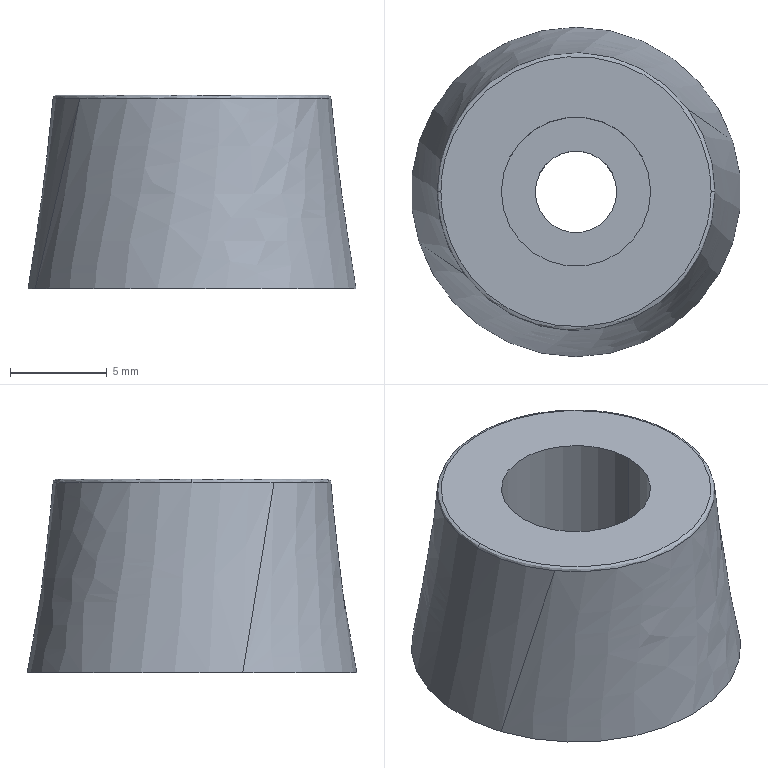Part | SolidWorks | features BaseBody 1 | 1 solid | 11 faces | box 17 x 17 x 10 mm | volume 1547 mm3 | spline 4 | cylinder 4 | plane 3 | commonest cylinder face diameters 4.2 x2 7.7 x2
STEP:
#1=CARTESIAN_POINT('',(6.967,0.,10.));
#2=VERTEX_POINT('',#1);
#3=CARTESIAN_POINT('',(-6.967,0.,10.));
#4=VERTEX_POINT('',#3);
#5=CARTESIAN_POINT('',(6.967,0.,10.));
#6=CARTESIAN_POINT('',(6.967,-13.935,10.));
#7=CARTESIAN_POINT('',(-6.967,-13.935,10.));
#8=CARTESIAN_POINT('',(-6.967,0.,10.));
#9=(BOUNDED_CURVE()B_SPLINE_CURVE(3,(#5,#6,#7,#8),.UNSPECIFIED.,.F.,.F.)B_SPLINE_CURVE_WITH_KNOTS((4,4),(0.,1.),.UNSPECIFIED.)CURVE()GEOMETRIC_REPRESENTATION_ITEM()RATIONAL_B_SPLINE_CURVE((1.,0.3333,0.3333,1.))REPRESENTATION_ITEM(''));
#10=EDGE_CURVE('',#2,#4,#9,.T.);
#11=ORIENTED_EDGE('',*,*,#10,.T.);
#12=CARTESIAN_POINT('',(-7.167,0.,9.818));
#13=VERTEX_POINT('',#12);
#14=CARTESIAN_POINT('',(-6.967,0.,9.8));
#15=DIRECTION('',(0.,-1.,0.));
#16=DIRECTION('',(-1.,0.,0.));
#17=AXIS2_PLACEMENT_3D('',#14,#15,#16);
#18=CIRCLE('',#17,0.2);
#19=EDGE_CURVE('',#4,#13,#18,.T.);
#20=ORIENTED_EDGE('',*,*,#19,.T.);
#21=CARTESIAN_POINT('',(-5.784,-4.231,9.818));
#22=VERTEX_POINT('',#21);
#23=CARTESIAN_POINT('',(0.,0.,9.818));
#24=DIRECTION('',(0.,0.,-1.));
#25=DIRECTION('',(-0.8071,-0.5904,0.));
#26=AXIS2_PLACEMENT_3D('',#23,#24,#25);
#27=CIRCLE('',#26,7.167);
#28=EDGE_CURVE('',#22,#13,#27,.T.);
#29=ORIENTED_EDGE('',*,*,#28,.F.);
#30=CARTESIAN_POINT('',(7.167,0.,9.818));
#31=VERTEX_POINT('',#30);
#32=CARTESIAN_POINT('',(0.,0.,9.818));
#33=DIRECTION('',(0.,0.,-1.));
#34=DIRECTION('',(-0.8071,-0.5904,0.));
#35=AXIS2_PLACEMENT_3D('',#32,#33,#34);
#36=CIRCLE('',#35,7.167);
#37=EDGE_CURVE('',#31,#22,#36,.T.);
#38=ORIENTED_EDGE('',*,*,#37,.F.);
#39=CARTESIAN_POINT('',(6.967,0.,9.8));
#40=DIRECTION('',(0.,1.,0.));
#41=DIRECTION('',(1.,0.,0.));
#42=AXIS2_PLACEMENT_3D('',#39,#40,#41);
#43=CIRCLE('',#42,0.2);
#44=EDGE_CURVE('',#2,#31,#43,.T.);
#45=ORIENTED_EDGE('',*,*,#44,.F.);
#46=EDGE_LOOP('',(#11,#20,#29,#38,#45));
#47=FACE_OUTER_BOUND('',#46,.T.);
#48=CARTESIAN_POINT('',(-6.967,0.,10.));
#49=CARTESIAN_POINT('',(-6.967,-13.935,10.));
#50=CARTESIAN_POINT('',(6.967,-13.935,10.));
#51=CARTESIAN_POINT('',(6.967,0.,10.));
#52=CARTESIAN_POINT('',(-7.076,0.,10.));
#53=CARTESIAN_POINT('',(-7.076,-14.152,10.));
#54=CARTESIAN_POINT('',(7.076,-14.152,10.));
#55=CARTESIAN_POINT('',(7.076,0.,10.));
#56=CARTESIAN_POINT('',(-7.157,0.,9.927));
#57=CARTESIAN_POINT('',(-7.157,-14.313,9.927));
#58=CARTESIAN_POINT('',(7.157,-14.313,9.927));
#59=CARTESIAN_POINT('',(7.157,0.,9.927));
#60=CARTESIAN_POINT('',(-7.167,0.,9.818));
#61=CARTESIAN_POINT('',(-7.167,-14.333,9.818));
#62=CARTESIAN_POINT('',(7.167,-14.333,9.818));
#63=CARTESIAN_POINT('',(7.167,0.,9.818));
#64=(BOUNDED_SURFACE()B_SPLINE_SURFACE(3,3,((#48,#49,#50,#51),(#52,#53,#54,#55),(#56,#57,#58,#59),(#60,#61,#62,#63)),.UNSPECIFIED.,.F.,.F.,.F.)B_SPLINE_SURFACE_WITH_KNOTS((4,4),(4,4),(0.,1.),(0.,1.),.UNSPECIFIED.)GEOMETRIC_REPRESENTATION_ITEM()RATIONAL_B_SPLINE_SURFACE(((1.,0.3333,0.3333,1.),(0.8259,0.2753,0.2753,0.8259),(0.8259,0.2753,0.2753,0.8259),(1.,0.3333,0.3333,1.)))REPRESENTATION_ITEM('')SURFACE());
#65=ADVANCED_FACE('',(#47),#64,.T.);
#66=CARTESIAN_POINT('',(-8.086,-2.622,0.));
#67=VERTEX_POINT('',#66);
#68=CARTESIAN_POINT('',(8.086,2.622,0.));
#69=VERTEX_POINT('',#68);
#70=CARTESIAN_POINT('',(0.,0.,0.));
#71=DIRECTION('',(0.,0.,1.));
#72=DIRECTION('',(1.,0.,0.));
#73=AXIS2_PLACEMENT_3D('',#70,#71,#72);
#74=CIRCLE('',#73,8.5);
#75=EDGE_CURVE('',#67,#69,#74,.T.);
#76=ORIENTED_EDGE('',*,*,#75,.T.);
#77=CARTESIAN_POINT('',(5.784,4.231,9.818));
#78=VERTEX_POINT('',#77);
#79=CARTESIAN_POINT('',(8.086,2.622,0.));
#80=CARTESIAN_POINT('',(5.784,4.231,9.818));
#81=B_SPLINE_CURVE_WITH_KNOTS('',1,(#79,#80),.UNSPECIFIED.,.F.,.F.,(2,2),(0.,0.9818),.UNSPECIFIED.);
#82=EDGE_CURVE('',#69,#78,#81,.T.);
#83=ORIENTED_EDGE('',*,*,#82,.T.);
#84=CARTESIAN_POINT('',(0.,0.,9.818));
#85=DIRECTION('',(0.,0.,-1.));
#86=DIRECTION('',(-0.8071,-0.5904,0.));
#87=AXIS2_PLACEMENT_3D('',#84,#85,#86);
#88=CIRCLE('',#87,7.167);
#89=EDGE_CURVE('',#78,#31,#88,.T.);
#90=ORIENTED_EDGE('',*,*,#89,.T.);
#91=ORIENTED_EDGE('',*,*,#37,.T.);
#92=CARTESIAN_POINT('',(-8.086,-2.622,0.));
#93=CARTESIAN_POINT('',(-5.784,-4.231,9.818));
#94=B_SPLINE_CURVE_WITH_KNOTS('',1,(#92,#93),.UNSPECIFIED.,.F.,.F.,(2,2),(0.,0.9818),.UNSPECIFIED.);
#95=EDGE_CURVE('',#67,#22,#94,.T.);
#96=ORIENTED_EDGE('',*,*,#95,.F.);
#97=EDGE_LOOP('',(#76,#83,#90,#91,#96));
#98=FACE_OUTER_BOUND('',#97,.T.);
#99=CARTESIAN_POINT('',(-8.086,-2.622,0.));
#100=CARTESIAN_POINT('',(-5.742,-4.261,10.));
#101=CARTESIAN_POINT('',(-2.842,-18.793,0.));
#102=CARTESIAN_POINT('',(2.779,-15.744,10.));
#103=CARTESIAN_POINT('',(13.329,-13.55,0.));
#104=CARTESIAN_POINT('',(14.263,-7.223,10.));
#105=CARTESIAN_POINT('',(8.086,2.622,0.));
#106=CARTESIAN_POINT('',(5.742,4.261,10.));
#107=CARTESIAN_POINT('',(2.842,18.793,0.));
#108=CARTESIAN_POINT('',(-2.779,15.744,10.));
#109=CARTESIAN_POINT('',(-13.329,13.55,0.));
#110=CARTESIAN_POINT('',(-14.263,7.223,10.));
#111=CARTESIAN_POINT('',(-8.086,-2.622,0.));
#112=CARTESIAN_POINT('',(-5.742,-4.261,10.));
#113=(BOUNDED_SURFACE()B_SPLINE_SURFACE(3,1,((#99,#100),(#101,#102),(#103,#104),(#105,#106),(#107,#108),(#109,#110),(#111,#112)),.UNSPECIFIED.,.T.,.F.,.F.)B_SPLINE_SURFACE_WITH_KNOTS((4,3,4),(2,2),(0.,0.5,1.),(0.,1.),.UNSPECIFIED.)GEOMETRIC_REPRESENTATION_ITEM()RATIONAL_B_SPLINE_SURFACE(((1.,1.),(0.3333,0.3333),(0.3333,0.3333),(1.,1.),(0.3333,0.3333),(0.3333,0.3333),(1.,1.)))REPRESENTATION_ITEM('')SURFACE());
#114=ADVANCED_FACE('',(#98),#113,.T.);
#115=CARTESIAN_POINT('',(2.1,0.,0.));
#116=VERTEX_POINT('',#115);
#117=CARTESIAN_POINT('',(-2.1,0.,0.));
#118=VERTEX_POINT('',#117);
#119=CARTESIAN_POINT('',(0.,0.,0.));
#120=DIRECTION('',(0.,0.,-1.));
#121=DIRECTION('',(1.,0.,0.));
#122=AXIS2_PLACEMENT_3D('',#119,#120,#121);
#123=CIRCLE('',#122,2.1);
#124=EDGE_CURVE('',#116,#118,#123,.T.);
#125=ORIENTED_EDGE('',*,*,#124,.T.);
#126=CARTESIAN_POINT('',(-2.1,0.,3.6));
#127=VERTEX_POINT('',#126);
#128=CARTESIAN_POINT('',(-2.1,0.,-2.8));
#129=DIRECTION('',(0.,0.,1.));
#130=VECTOR('',#129,1000.);
#131=LINE('',#128,#130);
#132=EDGE_CURVE('',#118,#127,#131,.T.);
#133=ORIENTED_EDGE('',*,*,#132,.T.);
#134=CARTESIAN_POINT('',(2.1,0.,3.6));
#135=VERTEX_POINT('',#134);
#136=CARTESIAN_POINT('',(0.,0.,3.6));
#137=DIRECTION('',(0.,0.,-1.));
#138=DIRECTION('',(1.,0.,0.));
#139=AXIS2_PLACEMENT_3D('',#136,#137,#138);
#140=CIRCLE('',#139,2.1);
#141=EDGE_CURVE('',#135,#127,#140,.T.);
#142=ORIENTED_EDGE('',*,*,#141,.F.);
#143=CARTESIAN_POINT('',(2.1,0.,-2.8));
#144=DIRECTION('',(0.,0.,1.));
#145=VECTOR('',#144,1000.);
#146=LINE('',#143,#145);
#147=EDGE_CURVE('',#116,#135,#146,.T.);
#148=ORIENTED_EDGE('',*,*,#147,.F.);
#149=EDGE_LOOP('',(#125,#133,#142,#148));
#150=FACE_OUTER_BOUND('',#149,.T.);
#151=CARTESIAN_POINT('',(0.,0.,-2.8));
#152=DIRECTION('',(0.,0.,1.));
#153=DIRECTION('',(1.,0.,0.));
#154=AXIS2_PLACEMENT_3D('',#151,#152,#153);
#155=CYLINDRICAL_SURFACE('',#154,2.1);
#156=ADVANCED_FACE('',(#150),#155,.F.);
#157=CARTESIAN_POINT('',(-3.85,0.,3.6));
#158=VERTEX_POINT('',#157);
#159=CARTESIAN_POINT('',(3.85,0.,3.6));
#160=VERTEX_POINT('',#159);
#161=CARTESIAN_POINT('',(0.,0.,3.6));
#162=DIRECTION('',(0.,0.,1.));
#163=DIRECTION('',(1.,0.,0.));
#164=AXIS2_PLACEMENT_3D('',#161,#162,#163);
#165=CIRCLE('',#164,3.85);
#166=EDGE_CURVE('',#158,#160,#165,.T.);
#167=ORIENTED_EDGE('',*,*,#166,.F.);
#168=CARTESIAN_POINT('',(-3.85,0.,10.));
#169=VERTEX_POINT('',#168);
#170=CARTESIAN_POINT('',(-3.85,0.,3.6));
#171=DIRECTION('',(0.,0.,1.));
#172=VECTOR('',#171,1000.);
#173=LINE('',#170,#172);
#174=EDGE_CURVE('',#158,#169,#173,.T.);
#175=ORIENTED_EDGE('',*,*,#174,.T.);
#176=CARTESIAN_POINT('',(3.85,0.,10.));
#177=VERTEX_POINT('',#176);
#178=CARTESIAN_POINT('',(0.,0.,10.));
#179=DIRECTION('',(0.,0.,-1.));
#180=DIRECTION('',(1.,0.,0.));
#181=AXIS2_PLACEMENT_3D('',#178,#179,#180);
#182=CIRCLE('',#181,3.85);
#183=EDGE_CURVE('',#177,#169,#182,.T.);
#184=ORIENTED_EDGE('',*,*,#183,.F.);
#185=CARTESIAN_POINT('',(3.85,0.,3.6));
#186=DIRECTION('',(0.,0.,1.));
#187=VECTOR('',#186,1000.);
#188=LINE('',#185,#187);
#189=EDGE_CURVE('',#160,#177,#188,.T.);
#190=ORIENTED_EDGE('',*,*,#189,.F.);
#191=EDGE_LOOP('',(#167,#175,#184,#190));
#192=FACE_OUTER_BOUND('',#191,.T.);
#193=CARTESIAN_POINT('',(0.,0.,3.6));
#194=DIRECTION('',(0.,0.,1.));
#195=DIRECTION('',(1.,0.,0.));
#196=AXIS2_PLACEMENT_3D('',#193,#194,#195);
#197=CYLINDRICAL_SURFACE('',#196,3.85);
#198=ADVANCED_FACE('',(#192),#197,.F.);
#199=ORIENTED_EDGE('',*,*,#82,.F.);
#200=CARTESIAN_POINT('',(0.,0.,0.));
#201=DIRECTION('',(0.,0.,1.));
#202=DIRECTION('',(1.,0.,0.));
#203=AXIS2_PLACEMENT_3D('',#200,#201,#202);
#204=CIRCLE('',#203,8.5);
#205=EDGE_CURVE('',#69,#67,#204,.T.);
#206=ORIENTED_EDGE('',*,*,#205,.T.);
#207=ORIENTED_EDGE('',*,*,#95,.T.);
#208=ORIENTED_EDGE('',*,*,#28,.T.);
#209=CARTESIAN_POINT('',(0.,0.,9.818));
#210=DIRECTION('',(0.,0.,-1.));
#211=DIRECTION('',(-0.8071,-0.5904,0.));
#212=AXIS2_PLACEMENT_3D('',#209,#210,#211);
#213=CIRCLE('',#212,7.167);
#214=EDGE_CURVE('',#13,#78,#213,.T.);
#215=ORIENTED_EDGE('',*,*,#214,.T.);
#216=EDGE_LOOP('',(#199,#206,#207,#208,#215));
#217=FACE_OUTER_BOUND('',#216,.T.);
#218=CARTESIAN_POINT('',(-8.086,-2.622,0.));
#219=CARTESIAN_POINT('',(-5.742,-4.261,10.));
#220=CARTESIAN_POINT('',(-2.842,-18.793,0.));
#221=CARTESIAN_POINT('',(2.779,-15.744,10.));
#222=CARTESIAN_POINT('',(13.329,-13.55,0.));
#223=CARTESIAN_POINT('',(14.263,-7.223,10.));
#224=CARTESIAN_POINT('',(8.086,2.622,0.));
#225=CARTESIAN_POINT('',(5.742,4.261,10.));
#226=CARTESIAN_POINT('',(2.842,18.793,0.));
#227=CARTESIAN_POINT('',(-2.779,15.744,10.));
#228=CARTESIAN_POINT('',(-13.329,13.55,0.));
#229=CARTESIAN_POINT('',(-14.263,7.223,10.));
#230=CARTESIAN_POINT('',(-8.086,-2.622,0.));
#231=CARTESIAN_POINT('',(-5.742,-4.261,10.));
#232=(BOUNDED_SURFACE()B_SPLINE_SURFACE(3,1,((#218,#219),(#220,#221),(#222,#223),(#224,#225),(#226,#227),(#228,#229),(#230,#231)),.UNSPECIFIED.,.T.,.F.,.F.)B_SPLINE_SURFACE_WITH_KNOTS((4,3,4),(2,2),(0.,0.5,1.),(0.,1.),.UNSPECIFIED.)GEOMETRIC_REPRESENTATION_ITEM()RATIONAL_B_SPLINE_SURFACE(((1.,1.),(0.3333,0.3333),(0.3333,0.3333),(1.,1.),(0.3333,0.3333),(0.3333,0.3333),(1.,1.)))REPRESENTATION_ITEM('')SURFACE());
#233=ADVANCED_FACE('',(#217),#232,.T.);
#234=ORIENTED_EDGE('',*,*,#19,.F.);
#235=CARTESIAN_POINT('',(-6.967,0.,10.));
#236=CARTESIAN_POINT('',(-6.967,13.935,10.));
#237=CARTESIAN_POINT('',(6.967,13.935,10.));
#238=CARTESIAN_POINT('',(6.967,0.,10.));
#239=(BOUNDED_CURVE()B_SPLINE_CURVE(3,(#235,#236,#237,#238),.UNSPECIFIED.,.F.,.F.)B_SPLINE_CURVE_WITH_KNOTS((4,4),(0.,1.),.UNSPECIFIED.)CURVE()GEOMETRIC_REPRESENTATION_ITEM()RATIONAL_B_SPLINE_CURVE((1.,0.3333,0.3333,1.))REPRESENTATION_ITEM(''));
#240=EDGE_CURVE('',#4,#2,#239,.T.);
#241=ORIENTED_EDGE('',*,*,#240,.T.);
#242=ORIENTED_EDGE('',*,*,#44,.T.);
#243=ORIENTED_EDGE('',*,*,#89,.F.);
#244=ORIENTED_EDGE('',*,*,#214,.F.);
#245=EDGE_LOOP('',(#234,#241,#242,#243,#244));
#246=FACE_OUTER_BOUND('',#245,.T.);
#247=CARTESIAN_POINT('',(6.967,0.,10.));
#248=CARTESIAN_POINT('',(6.967,13.935,10.));
#249=CARTESIAN_POINT('',(-6.967,13.935,10.));
#250=CARTESIAN_POINT('',(-6.967,0.,10.));
#251=CARTESIAN_POINT('',(7.076,0.,10.));
#252=CARTESIAN_POINT('',(7.076,14.152,10.));
#253=CARTESIAN_POINT('',(-7.076,14.152,10.));
#254=CARTESIAN_POINT('',(-7.076,0.,10.));
#255=CARTESIAN_POINT('',(7.157,0.,9.927));
#256=CARTESIAN_POINT('',(7.157,14.313,9.927));
#257=CARTESIAN_POINT('',(-7.157,14.313,9.927));
#258=CARTESIAN_POINT('',(-7.157,0.,9.927));
#259=CARTESIAN_POINT('',(7.167,0.,9.818));
#260=CARTESIAN_POINT('',(7.167,14.333,9.818));
#261=CARTESIAN_POINT('',(-7.167,14.333,9.818));
#262=CARTESIAN_POINT('',(-7.167,0.,9.818));
#263=(BOUNDED_SURFACE()B_SPLINE_SURFACE(3,3,((#247,#248,#249,#250),(#251,#252,#253,#254),(#255,#256,#257,#258),(#259,#260,#261,#262)),.UNSPECIFIED.,.F.,.F.,.F.)B_SPLINE_SURFACE_WITH_KNOTS((4,4),(4,4),(0.,1.),(0.,1.),.UNSPECIFIED.)GEOMETRIC_REPRESENTATION_ITEM()RATIONAL_B_SPLINE_SURFACE(((1.,0.3333,0.3333,1.),(0.8259,0.2753,0.2753,0.8259),(0.8259,0.2753,0.2753,0.8259),(1.,0.3333,0.3333,1.)))REPRESENTATION_ITEM('')SURFACE());
#264=ADVANCED_FACE('',(#246),#263,.T.);
#265=ORIENTED_EDGE('',*,*,#75,.F.);
#266=ORIENTED_EDGE('',*,*,#205,.F.);
#267=EDGE_LOOP('',(#265,#266));
#268=FACE_OUTER_BOUND('',#267,.T.);
#269=ORIENTED_EDGE('',*,*,#124,.F.);
#270=CARTESIAN_POINT('',(0.,0.,0.));
#271=DIRECTION('',(0.,0.,-1.));
#272=DIRECTION('',(1.,0.,0.));
#273=AXIS2_PLACEMENT_3D('',#270,#271,#272);
#274=CIRCLE('',#273,2.1);
#275=EDGE_CURVE('',#118,#116,#274,.T.);
#276=ORIENTED_EDGE('',*,*,#275,.F.);
#277=EDGE_LOOP('',(#269,#276));
#278=FACE_BOUND('',#277,.T.);
#279=CARTESIAN_POINT('',(0.,0.,0.));
#280=DIRECTION('',(0.,0.,1.));
#281=DIRECTION('',(1.,0.,0.));
#282=AXIS2_PLACEMENT_3D('',#279,#280,#281);
#283=PLANE('',#282);
#284=ADVANCED_FACE('',(#268,#278),#283,.F.);
#285=ORIENTED_EDGE('',*,*,#183,.T.);
#286=CARTESIAN_POINT('',(0.,0.,10.));
#287=DIRECTION('',(0.,0.,-1.));
#288=DIRECTION('',(1.,0.,0.));
#289=AXIS2_PLACEMENT_3D('',#286,#287,#288);
#290=CIRCLE('',#289,3.85);
#291=EDGE_CURVE('',#169,#177,#290,.T.);
#292=ORIENTED_EDGE('',*,*,#291,.T.);
#293=EDGE_LOOP('',(#285,#292));
#294=FACE_BOUND('',#293,.T.);
#295=ORIENTED_EDGE('',*,*,#240,.F.);
#296=ORIENTED_EDGE('',*,*,#10,.F.);
#297=EDGE_LOOP('',(#295,#296));
#298=FACE_OUTER_BOUND('',#297,.T.);
#299=CARTESIAN_POINT('',(0.,0.,10.));
#300=DIRECTION('',(0.,0.,1.));
#301=DIRECTION('',(1.,0.,0.));
#302=AXIS2_PLACEMENT_3D('',#299,#300,#301);
#303=PLANE('',#302);
#304=ADVANCED_FACE('',(#294,#298),#303,.T.);
#305=ORIENTED_EDGE('',*,*,#132,.F.);
#306=ORIENTED_EDGE('',*,*,#275,.T.);
#307=ORIENTED_EDGE('',*,*,#147,.T.);
#308=CARTESIAN_POINT('',(0.,0.,3.6));
#309=DIRECTION('',(0.,0.,-1.));
#310=DIRECTION('',(1.,0.,0.));
#311=AXIS2_PLACEMENT_3D('',#308,#309,#310);
#312=CIRCLE('',#311,2.1);
#313=EDGE_CURVE('',#127,#135,#312,.T.);
#314=ORIENTED_EDGE('',*,*,#313,.F.);
#315=EDGE_LOOP('',(#305,#306,#307,#314));
#316=FACE_OUTER_BOUND('',#315,.T.);
#317=CARTESIAN_POINT('',(0.,0.,-2.8));
#318=DIRECTION('',(0.,0.,1.));
#319=DIRECTION('',(1.,0.,0.));
#320=AXIS2_PLACEMENT_3D('',#317,#318,#319);
#321=CYLINDRICAL_SURFACE('',#320,2.1);
#322=ADVANCED_FACE('',(#316),#321,.F.);
#323=ORIENTED_EDGE('',*,*,#174,.F.);
#324=CARTESIAN_POINT('',(0.,0.,3.6));
#325=DIRECTION('',(0.,0.,1.));
#326=DIRECTION('',(1.,0.,0.));
#327=AXIS2_PLACEMENT_3D('',#324,#325,#326);
#328=CIRCLE('',#327,3.85);
#329=EDGE_CURVE('',#160,#158,#328,.T.);
#330=ORIENTED_EDGE('',*,*,#329,.F.);
#331=ORIENTED_EDGE('',*,*,#189,.T.);
#332=ORIENTED_EDGE('',*,*,#291,.F.);
#333=EDGE_LOOP('',(#323,#330,#331,#332));
#334=FACE_OUTER_BOUND('',#333,.T.);
#335=CARTESIAN_POINT('',(0.,0.,3.6));
#336=DIRECTION('',(0.,0.,1.));
#337=DIRECTION('',(1.,0.,0.));
#338=AXIS2_PLACEMENT_3D('',#335,#336,#337);
#339=CYLINDRICAL_SURFACE('',#338,3.85);
#340=ADVANCED_FACE('',(#334),#339,.F.);
#341=ORIENTED_EDGE('',*,*,#329,.T.);
#342=ORIENTED_EDGE('',*,*,#166,.T.);
#343=EDGE_LOOP('',(#341,#342));
#344=FACE_OUTER_BOUND('',#343,.T.);
#345=ORIENTED_EDGE('',*,*,#141,.T.);
#346=ORIENTED_EDGE('',*,*,#313,.T.);
#347=EDGE_LOOP('',(#345,#346));
#348=FACE_BOUND('',#347,.T.);
#349=CARTESIAN_POINT('',(0.,0.,3.6));
#350=DIRECTION('',(0.,0.,1.));
#351=DIRECTION('',(1.,0.,0.));
#352=AXIS2_PLACEMENT_3D('',#349,#350,#351);
#353=PLANE('',#352);
#354=ADVANCED_FACE('',(#344,#348),#353,.T.);
#355=CLOSED_SHELL('',(#65,#114,#156,#198,#233,#264,#284,#304,#322,#340,#354));
#356=MANIFOLD_SOLID_BREP('',#355);
#357=CARTESIAN_POINT('',(0.,0.,0.));
#358=DIRECTION('',(0.,0.,1.));
#359=DIRECTION('',(1.,0.,0.));
#360=AXIS2_PLACEMENT_3D('',#357,#358,#359);
#361=(LENGTH_UNIT()NAMED_UNIT(*)SI_UNIT(.MILLI.,.METRE.));
#362=UNCERTAINTY_MEASURE_WITH_UNIT(LENGTH_MEASURE(0.00001),#361,'','');
#363=(NAMED_UNIT(*)PLANE_ANGLE_UNIT()SI_UNIT($,.RADIAN.));
#364=(NAMED_UNIT(*)SI_UNIT($,.STERADIAN.)SOLID_ANGLE_UNIT());
#365=(GEOMETRIC_REPRESENTATION_CONTEXT(3)GLOBAL_UNCERTAINTY_ASSIGNED_CONTEXT((#362))GLOBAL_UNIT_ASSIGNED_CONTEXT((#361,#363,#364))REPRESENTATION_CONTEXT('',''));
#366=ADVANCED_BREP_SHAPE_REPRESENTATION('',(#356,#360),#365);